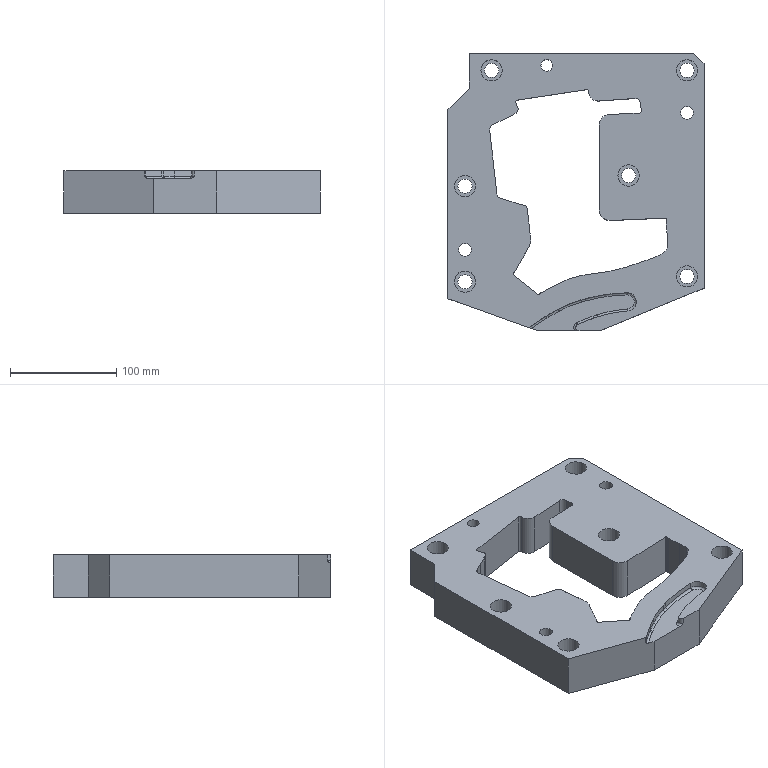Part | NX | features 23 2 | 1 solid | 113 faces | box 241 x 261 x 40 mm | volume 1551102 mm3 | cylinder 53 | plane 38 | spline 18 | torus 4 | commonest cylinder face diameters 2 x9 20 x8 13.5 x6 10 x3 3 x2 12.001 x2